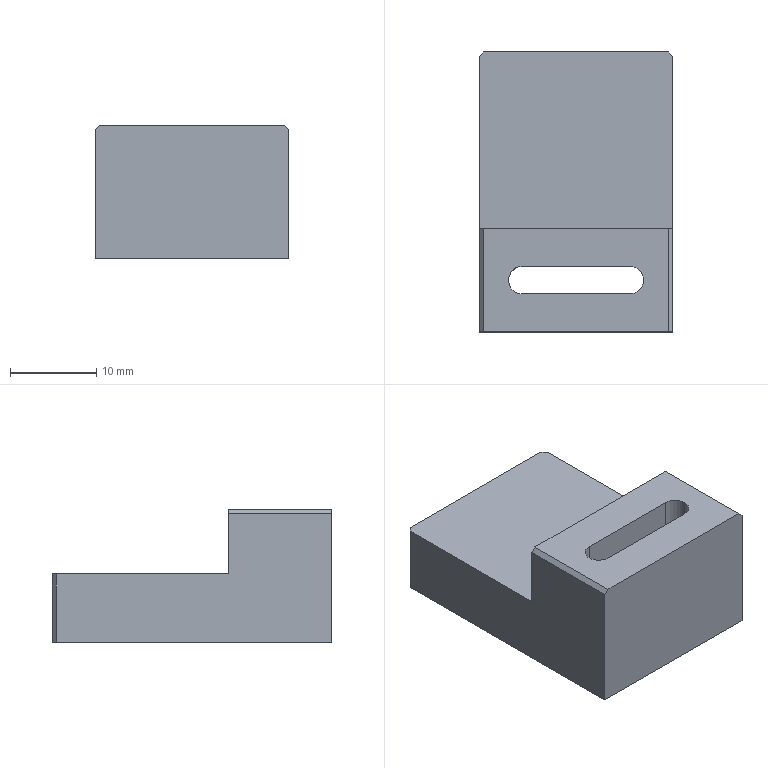Part | STEP file | PN_0033 | 1 solid | 33 faces | box 22.5 x 32.5 x 15.5 mm | volume 7082 mm3 | plane 14 | cylinder 11 | cone 8 | commonest cylinder face diameters 1.6 x8 3.2 x3